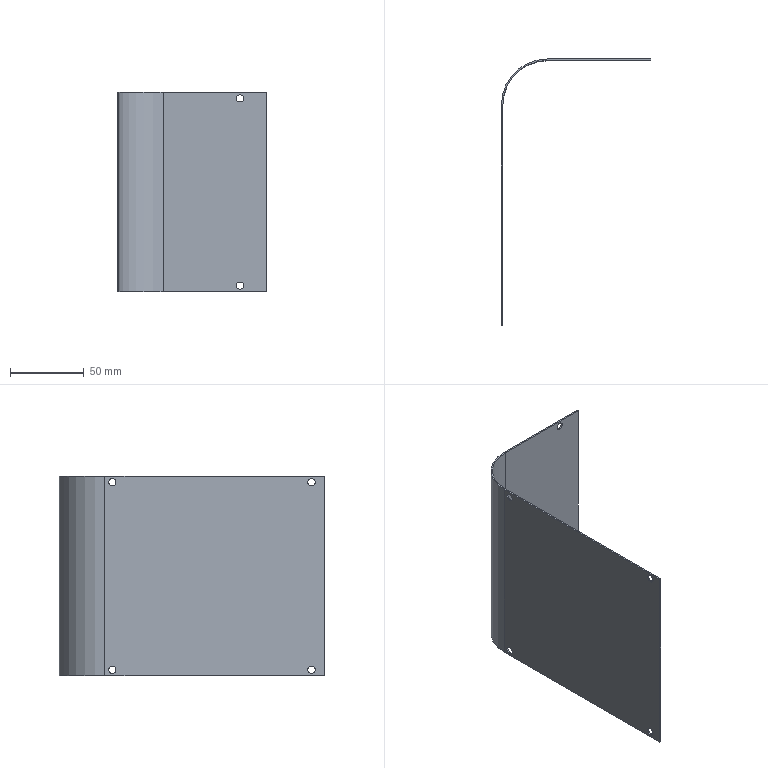Part | NX | 1 solid | 20 faces | box 101 x 180 x 135 mm | volume 35915 mm3 | plane 12 | cylinder 8 | commonest cylinder face diameters 5 x6 60 x1 62 x1
STEP:
#1=CARTESIAN_POINT('',(0.,-30.,67.5));
#2=VERTEX_POINT('',#1);
#3=CARTESIAN_POINT('',(-1.,-30.,67.5));
#4=VERTEX_POINT('',#3);
#5=CARTESIAN_POINT('',(0.,-30.,67.5));
#6=DIRECTION('',(-1.,0.,0.));
#7=VECTOR('',#6,1000.);
#8=LINE('',#5,#7);
#9=EDGE_CURVE('',#2,#4,#8,.T.);
#10=ORIENTED_EDGE('',*,*,#9,.F.);
#11=CARTESIAN_POINT('',(30.,0.,67.5));
#12=VERTEX_POINT('',#11);
#13=CARTESIAN_POINT('',(30.,-30.,67.5));
#14=DIRECTION('',(0.,0.,1.));
#15=DIRECTION('',(-1.,0.,0.));
#16=AXIS2_PLACEMENT_3D('',#13,#14,#15);
#17=CIRCLE('',#16,30.);
#18=EDGE_CURVE('',#12,#2,#17,.T.);
#19=ORIENTED_EDGE('',*,*,#18,.F.);
#20=CARTESIAN_POINT('',(30.,1.,67.5));
#21=VERTEX_POINT('',#20);
#22=CARTESIAN_POINT('',(30.,1.,67.5));
#23=DIRECTION('',(0.,-1.,0.));
#24=VECTOR('',#23,1000.);
#25=LINE('',#22,#24);
#26=EDGE_CURVE('',#21,#12,#25,.T.);
#27=ORIENTED_EDGE('',*,*,#26,.F.);
#28=CARTESIAN_POINT('',(30.,-30.,67.5));
#29=DIRECTION('',(0.,0.,1.));
#30=DIRECTION('',(1.,0.,0.));
#31=AXIS2_PLACEMENT_3D('',#28,#29,#30);
#32=CIRCLE('',#31,31.);
#33=EDGE_CURVE('',#21,#4,#32,.T.);
#34=ORIENTED_EDGE('',*,*,#33,.T.);
#35=EDGE_LOOP('',(#10,#19,#27,#34));
#36=FACE_BOUND('',#35,.T.);
#37=CARTESIAN_POINT('',(0.,-30.,67.5));
#38=DIRECTION('',(0.,0.,1.));
#39=DIRECTION('',(1.,0.,0.));
#40=AXIS2_PLACEMENT_3D('',#37,#38,#39);
#41=PLANE('',#40);
#42=ADVANCED_FACE('',(#36),#41,.T.);
#43=CARTESIAN_POINT('',(0.,-179.,67.5));
#44=VERTEX_POINT('',#43);
#45=CARTESIAN_POINT('',(0.,-30.,67.5));
#46=DIRECTION('',(0.,-1.,0.));
#47=VECTOR('',#46,1000.);
#48=LINE('',#45,#47);
#49=EDGE_CURVE('',#2,#44,#48,.T.);
#50=ORIENTED_EDGE('',*,*,#49,.F.);
#51=ORIENTED_EDGE('',*,*,#9,.T.);
#52=CARTESIAN_POINT('',(-1.,-179.,67.5));
#53=VERTEX_POINT('',#52);
#54=CARTESIAN_POINT('',(-1.,-30.,67.5));
#55=DIRECTION('',(0.,-1.,0.));
#56=VECTOR('',#55,1000.);
#57=LINE('',#54,#56);
#58=EDGE_CURVE('',#4,#53,#57,.T.);
#59=ORIENTED_EDGE('',*,*,#58,.T.);
#60=CARTESIAN_POINT('',(0.,-179.,67.5));
#61=DIRECTION('',(-1.,0.,0.));
#62=VECTOR('',#61,1000.);
#63=LINE('',#60,#62);
#64=EDGE_CURVE('',#44,#53,#63,.T.);
#65=ORIENTED_EDGE('',*,*,#64,.F.);
#66=EDGE_LOOP('',(#50,#51,#59,#65));
#67=FACE_BOUND('',#66,.T.);
#68=CARTESIAN_POINT('',(30.,1.,67.5));
#69=DIRECTION('',(0.,0.,1.));
#70=DIRECTION('',(1.,0.,0.));
#71=AXIS2_PLACEMENT_3D('',#68,#69,#70);
#72=PLANE('',#71);
#73=ADVANCED_FACE('',(#67),#72,.T.);
#74=CARTESIAN_POINT('',(30.,0.,-67.5));
#75=VERTEX_POINT('',#74);
#76=CARTESIAN_POINT('',(30.,1.,-67.5));
#77=VERTEX_POINT('',#76);
#78=CARTESIAN_POINT('',(30.,0.,-67.5));
#79=DIRECTION('',(0.,1.,0.));
#80=VECTOR('',#79,1000.);
#81=LINE('',#78,#80);
#82=EDGE_CURVE('',#75,#77,#81,.T.);
#83=ORIENTED_EDGE('',*,*,#82,.F.);
#84=CARTESIAN_POINT('',(0.,-30.,-67.5));
#85=VERTEX_POINT('',#84);
#86=CARTESIAN_POINT('',(30.,-30.,-67.5));
#87=DIRECTION('',(0.,0.,1.));
#88=DIRECTION('',(-1.,0.,0.));
#89=AXIS2_PLACEMENT_3D('',#86,#87,#88);
#90=CIRCLE('',#89,30.);
#91=EDGE_CURVE('',#75,#85,#90,.T.);
#92=ORIENTED_EDGE('',*,*,#91,.T.);
#93=CARTESIAN_POINT('',(-1.,-30.,-67.5));
#94=VERTEX_POINT('',#93);
#95=CARTESIAN_POINT('',(-1.,-30.,-67.5));
#96=DIRECTION('',(1.,0.,0.));
#97=VECTOR('',#96,1000.);
#98=LINE('',#95,#97);
#99=EDGE_CURVE('',#94,#85,#98,.T.);
#100=ORIENTED_EDGE('',*,*,#99,.F.);
#101=CARTESIAN_POINT('',(30.,-30.,-67.5));
#102=DIRECTION('',(0.,0.,1.));
#103=DIRECTION('',(1.,0.,0.));
#104=AXIS2_PLACEMENT_3D('',#101,#102,#103);
#105=CIRCLE('',#104,31.);
#106=EDGE_CURVE('',#77,#94,#105,.T.);
#107=ORIENTED_EDGE('',*,*,#106,.F.);
#108=EDGE_LOOP('',(#83,#92,#100,#107));
#109=FACE_BOUND('',#108,.T.);
#110=CARTESIAN_POINT('',(30.,0.,-67.5));
#111=DIRECTION('',(0.,0.,-1.));
#112=DIRECTION('',(-1.,0.,0.));
#113=AXIS2_PLACEMENT_3D('',#110,#111,#112);
#114=PLANE('',#113);
#115=ADVANCED_FACE('',(#109),#114,.T.);
#116=CARTESIAN_POINT('',(100.,0.,-67.5));
#117=VERTEX_POINT('',#116);
#118=CARTESIAN_POINT('',(30.,0.,-67.5));
#119=DIRECTION('',(-1.,0.,0.));
#120=VECTOR('',#119,1000.);
#121=LINE('',#118,#120);
#122=EDGE_CURVE('',#117,#75,#121,.T.);
#123=ORIENTED_EDGE('',*,*,#122,.T.);
#124=ORIENTED_EDGE('',*,*,#82,.T.);
#125=CARTESIAN_POINT('',(100.,1.,-67.5));
#126=VERTEX_POINT('',#125);
#127=CARTESIAN_POINT('',(30.,1.,-67.5));
#128=DIRECTION('',(1.,0.,0.));
#129=VECTOR('',#128,1000.);
#130=LINE('',#127,#129);
#131=EDGE_CURVE('',#126,#77,#130,.F.);
#132=ORIENTED_EDGE('',*,*,#131,.F.);
#133=CARTESIAN_POINT('',(100.,1.,-67.5));
#134=DIRECTION('',(0.,-1.,0.));
#135=VECTOR('',#134,1000.);
#136=LINE('',#133,#135);
#137=EDGE_CURVE('',#126,#117,#136,.T.);
#138=ORIENTED_EDGE('',*,*,#137,.T.);
#139=EDGE_LOOP('',(#123,#124,#132,#138));
#140=FACE_BOUND('',#139,.T.);
#141=CARTESIAN_POINT('',(-1.,-30.,-67.5));
#142=DIRECTION('',(0.,0.,-1.));
#143=DIRECTION('',(-1.,0.,0.));
#144=AXIS2_PLACEMENT_3D('',#141,#142,#143);
#145=PLANE('',#144);
#146=ADVANCED_FACE('',(#140),#145,.T.);
#147=CARTESIAN_POINT('',(-1.,-32.5,63.5));
#148=VERTEX_POINT('',#147);
#149=CARTESIAN_POINT('',(-1.,-35.,63.5));
#150=DIRECTION('',(-1.,0.,0.));
#151=DIRECTION('',(0.,1.,0.));
#152=AXIS2_PLACEMENT_3D('',#149,#150,#151);
#153=CIRCLE('',#152,2.5);
#154=EDGE_CURVE('',#148,#148,#153,.T.);
#155=ORIENTED_EDGE('',*,*,#154,.F.);
#156=EDGE_LOOP('',(#155));
#157=FACE_BOUND('',#156,.T.);
#158=CARTESIAN_POINT('',(-1.,-37.5,-63.5));
#159=VERTEX_POINT('',#158);
#160=CARTESIAN_POINT('',(-1.,-35.,-63.5));
#161=DIRECTION('',(-1.,0.,0.));
#162=DIRECTION('',(0.,-1.,0.));
#163=AXIS2_PLACEMENT_3D('',#160,#161,#162);
#164=CIRCLE('',#163,2.5);
#165=EDGE_CURVE('',#159,#159,#164,.T.);
#166=ORIENTED_EDGE('',*,*,#165,.F.);
#167=EDGE_LOOP('',(#166));
#168=FACE_BOUND('',#167,.T.);
#169=CARTESIAN_POINT('',(-1.,-172.5,63.5));
#170=VERTEX_POINT('',#169);
#171=CARTESIAN_POINT('',(-1.,-170.,63.5));
#172=DIRECTION('',(-1.,0.,0.));
#173=DIRECTION('',(0.,-1.,0.));
#174=AXIS2_PLACEMENT_3D('',#171,#172,#173);
#175=CIRCLE('',#174,2.5);
#176=EDGE_CURVE('',#170,#170,#175,.T.);
#177=ORIENTED_EDGE('',*,*,#176,.F.);
#178=EDGE_LOOP('',(#177));
#179=FACE_BOUND('',#178,.T.);
#180=CARTESIAN_POINT('',(-1.,-172.5,-63.5));
#181=VERTEX_POINT('',#180);
#182=CARTESIAN_POINT('',(-1.,-170.,-63.5));
#183=DIRECTION('',(-1.,0.,0.));
#184=DIRECTION('',(0.,-1.,0.));
#185=AXIS2_PLACEMENT_3D('',#182,#183,#184);
#186=CIRCLE('',#185,2.5);
#187=EDGE_CURVE('',#181,#181,#186,.T.);
#188=ORIENTED_EDGE('',*,*,#187,.F.);
#189=EDGE_LOOP('',(#188));
#190=FACE_BOUND('',#189,.T.);
#191=CARTESIAN_POINT('',(-1.,-179.,-67.5));
#192=VERTEX_POINT('',#191);
#193=CARTESIAN_POINT('',(-1.,-30.,-67.5));
#194=DIRECTION('',(0.,-1.,0.));
#195=VECTOR('',#194,1000.);
#196=LINE('',#193,#195);
#197=EDGE_CURVE('',#94,#192,#196,.T.);
#198=ORIENTED_EDGE('',*,*,#197,.T.);
#199=CARTESIAN_POINT('',(-1.,-179.,67.5));
#200=DIRECTION('',(0.,0.,-1.));
#201=VECTOR('',#200,1000.);
#202=LINE('',#199,#201);
#203=EDGE_CURVE('',#53,#192,#202,.T.);
#204=ORIENTED_EDGE('',*,*,#203,.F.);
#205=ORIENTED_EDGE('',*,*,#58,.F.);
#206=CARTESIAN_POINT('',(-1.,-30.,67.5));
#207=DIRECTION('',(0.,0.,-1.));
#208=VECTOR('',#207,1000.);
#209=LINE('',#206,#208);
#210=EDGE_CURVE('',#4,#94,#209,.T.);
#211=ORIENTED_EDGE('',*,*,#210,.T.);
#212=EDGE_LOOP('',(#198,#204,#205,#211));
#213=FACE_BOUND('',#212,.T.);
#214=CARTESIAN_POINT('',(-1.,-30.,67.5));
#215=DIRECTION('',(1.,0.,0.));
#216=DIRECTION('',(0.,1.,0.));
#217=AXIS2_PLACEMENT_3D('',#214,#215,#216);
#218=PLANE('',#217);
#219=ADVANCED_FACE('',(#157,#168,#179,#190,#213),#218,.F.);
#220=CARTESIAN_POINT('',(0.,-179.,-67.5));
#221=VERTEX_POINT('',#220);
#222=CARTESIAN_POINT('',(0.,-179.,-67.5));
#223=DIRECTION('',(-1.,0.,0.));
#224=VECTOR('',#223,1000.);
#225=LINE('',#222,#224);
#226=EDGE_CURVE('',#221,#192,#225,.T.);
#227=ORIENTED_EDGE('',*,*,#226,.F.);
#228=CARTESIAN_POINT('',(0.,-179.,67.5));
#229=DIRECTION('',(0.,0.,-1.));
#230=VECTOR('',#229,1000.);
#231=LINE('',#228,#230);
#232=EDGE_CURVE('',#44,#221,#231,.T.);
#233=ORIENTED_EDGE('',*,*,#232,.F.);
#234=ORIENTED_EDGE('',*,*,#64,.T.);
#235=ORIENTED_EDGE('',*,*,#203,.T.);
#236=EDGE_LOOP('',(#227,#233,#234,#235));
#237=FACE_BOUND('',#236,.T.);
#238=CARTESIAN_POINT('',(0.,-179.,67.5));
#239=DIRECTION('',(0.,-1.,0.));
#240=DIRECTION('',(0.,0.,-1.));
#241=AXIS2_PLACEMENT_3D('',#238,#239,#240);
#242=PLANE('',#241);
#243=ADVANCED_FACE('',(#237),#242,.T.);
#244=CARTESIAN_POINT('',(0.,-32.5,63.5));
#245=VERTEX_POINT('',#244);
#246=CARTESIAN_POINT('',(0.,-35.,63.5));
#247=DIRECTION('',(1.,0.,0.));
#248=DIRECTION('',(0.,1.,0.));
#249=AXIS2_PLACEMENT_3D('',#246,#247,#248);
#250=CIRCLE('',#249,2.5);
#251=EDGE_CURVE('',#245,#245,#250,.T.);
#252=ORIENTED_EDGE('',*,*,#251,.F.);
#253=EDGE_LOOP('',(#252));
#254=FACE_BOUND('',#253,.T.);
#255=CARTESIAN_POINT('',(0.,-32.5,-63.5));
#256=VERTEX_POINT('',#255);
#257=CARTESIAN_POINT('',(0.,-35.,-63.5));
#258=DIRECTION('',(1.,0.,0.));
#259=DIRECTION('',(0.,1.,0.));
#260=AXIS2_PLACEMENT_3D('',#257,#258,#259);
#261=CIRCLE('',#260,2.5);
#262=EDGE_CURVE('',#256,#256,#261,.T.);
#263=ORIENTED_EDGE('',*,*,#262,.F.);
#264=EDGE_LOOP('',(#263));
#265=FACE_BOUND('',#264,.T.);
#266=CARTESIAN_POINT('',(0.,-167.5,63.5));
#267=VERTEX_POINT('',#266);
#268=CARTESIAN_POINT('',(0.,-170.,63.5));
#269=DIRECTION('',(1.,0.,0.));
#270=DIRECTION('',(0.,1.,0.));
#271=AXIS2_PLACEMENT_3D('',#268,#269,#270);
#272=CIRCLE('',#271,2.5);
#273=EDGE_CURVE('',#267,#267,#272,.T.);
#274=ORIENTED_EDGE('',*,*,#273,.F.);
#275=EDGE_LOOP('',(#274));
#276=FACE_BOUND('',#275,.T.);
#277=CARTESIAN_POINT('',(0.,-167.5,-63.5));
#278=VERTEX_POINT('',#277);
#279=CARTESIAN_POINT('',(0.,-170.,-63.5));
#280=DIRECTION('',(1.,0.,0.));
#281=DIRECTION('',(0.,1.,0.));
#282=AXIS2_PLACEMENT_3D('',#279,#280,#281);
#283=CIRCLE('',#282,2.5);
#284=EDGE_CURVE('',#278,#278,#283,.T.);
#285=ORIENTED_EDGE('',*,*,#284,.F.);
#286=EDGE_LOOP('',(#285));
#287=FACE_BOUND('',#286,.T.);
#288=CARTESIAN_POINT('',(0.,-30.,-67.5));
#289=DIRECTION('',(0.,-1.,0.));
#290=VECTOR('',#289,1000.);
#291=LINE('',#288,#290);
#292=EDGE_CURVE('',#85,#221,#291,.T.);
#293=ORIENTED_EDGE('',*,*,#292,.F.);
#294=CARTESIAN_POINT('',(0.,-30.,67.5));
#295=DIRECTION('',(0.,0.,-1.));
#296=VECTOR('',#295,1000.);
#297=LINE('',#294,#296);
#298=EDGE_CURVE('',#2,#85,#297,.T.);
#299=ORIENTED_EDGE('',*,*,#298,.F.);
#300=ORIENTED_EDGE('',*,*,#49,.T.);
#301=ORIENTED_EDGE('',*,*,#232,.T.);
#302=EDGE_LOOP('',(#293,#299,#300,#301));
#303=FACE_BOUND('',#302,.T.);
#304=CARTESIAN_POINT('',(0.,-30.,67.5));
#305=DIRECTION('',(1.,0.,0.));
#306=DIRECTION('',(0.,1.,0.));
#307=AXIS2_PLACEMENT_3D('',#304,#305,#306);
#308=PLANE('',#307);
#309=ADVANCED_FACE('',(#254,#265,#276,#287,#303),#308,.T.);
#310=ORIENTED_EDGE('',*,*,#91,.F.);
#311=CARTESIAN_POINT('',(30.,0.,67.5));
#312=DIRECTION('',(0.,0.,-1.));
#313=VECTOR('',#312,1000.);
#314=LINE('',#311,#313);
#315=EDGE_CURVE('',#12,#75,#314,.T.);
#316=ORIENTED_EDGE('',*,*,#315,.F.);
#317=ORIENTED_EDGE('',*,*,#18,.T.);
#318=ORIENTED_EDGE('',*,*,#298,.T.);
#319=EDGE_LOOP('',(#310,#316,#317,#318));
#320=FACE_BOUND('',#319,.T.);
#321=CARTESIAN_POINT('',(30.,-30.,67.5));
#322=DIRECTION('',(0.,0.,-1.));
#323=DIRECTION('',(-1.,0.,0.));
#324=AXIS2_PLACEMENT_3D('',#321,#322,#323);
#325=CYLINDRICAL_SURFACE('',#324,30.);
#326=ADVANCED_FACE('',(#320),#325,.F.);
#327=CARTESIAN_POINT('',(82.,0.,61.));
#328=VERTEX_POINT('',#327);
#329=CARTESIAN_POINT('',(82.,0.,63.5));
#330=DIRECTION('',(0.,-1.,0.));
#331=DIRECTION('',(0.,0.,-1.));
#332=AXIS2_PLACEMENT_3D('',#329,#330,#331);
#333=CIRCLE('',#332,2.5);
#334=EDGE_CURVE('',#328,#328,#333,.T.);
#335=ORIENTED_EDGE('',*,*,#334,.F.);
#336=EDGE_LOOP('',(#335));
#337=FACE_BOUND('',#336,.T.);
#338=CARTESIAN_POINT('',(82.,0.,-66.));
#339=VERTEX_POINT('',#338);
#340=CARTESIAN_POINT('',(82.,0.,-63.5));
#341=DIRECTION('',(0.,-1.,0.));
#342=DIRECTION('',(0.,0.,-1.));
#343=AXIS2_PLACEMENT_3D('',#340,#341,#342);
#344=CIRCLE('',#343,2.5);
#345=EDGE_CURVE('',#339,#339,#344,.T.);
#346=ORIENTED_EDGE('',*,*,#345,.F.);
#347=EDGE_LOOP('',(#346));
#348=FACE_BOUND('',#347,.T.);
#349=ORIENTED_EDGE('',*,*,#122,.F.);
#350=CARTESIAN_POINT('',(100.,0.,67.5));
#351=VERTEX_POINT('',#350);
#352=CARTESIAN_POINT('',(100.,0.,67.5));
#353=DIRECTION('',(0.,0.,-1.));
#354=VECTOR('',#353,1000.);
#355=LINE('',#352,#354);
#356=EDGE_CURVE('',#351,#117,#355,.T.);
#357=ORIENTED_EDGE('',*,*,#356,.F.);
#358=CARTESIAN_POINT('',(30.,0.,67.5));
#359=DIRECTION('',(-1.,0.,0.));
#360=VECTOR('',#359,1000.);
#361=LINE('',#358,#360);
#362=EDGE_CURVE('',#351,#12,#361,.T.);
#363=ORIENTED_EDGE('',*,*,#362,.T.);
#364=ORIENTED_EDGE('',*,*,#315,.T.);
#365=EDGE_LOOP('',(#349,#357,#363,#364));
#366=FACE_BOUND('',#365,.T.);
#367=CARTESIAN_POINT('',(30.,0.,67.5));
#368=DIRECTION('',(0.,-1.,0.));
#369=DIRECTION('',(0.,0.,-1.));
#370=AXIS2_PLACEMENT_3D('',#367,#368,#369);
#371=PLANE('',#370);
#372=ADVANCED_FACE('',(#337,#348,#366),#371,.T.);
#373=ORIENTED_EDGE('',*,*,#137,.F.);
#374=CARTESIAN_POINT('',(100.,1.,67.5));
#375=VERTEX_POINT('',#374);
#376=CARTESIAN_POINT('',(100.,1.,67.5));
#377=DIRECTION('',(0.,0.,-1.));
#378=VECTOR('',#377,1000.);
#379=LINE('',#376,#378);
#380=EDGE_CURVE('',#375,#126,#379,.T.);
#381=ORIENTED_EDGE('',*,*,#380,.F.);
#382=CARTESIAN_POINT('',(100.,1.,67.5));
#383=DIRECTION('',(0.,-1.,0.));
#384=VECTOR('',#383,1000.);
#385=LINE('',#382,#384);
#386=EDGE_CURVE('',#375,#351,#385,.T.);
#387=ORIENTED_EDGE('',*,*,#386,.T.);
#388=ORIENTED_EDGE('',*,*,#356,.T.);
#389=EDGE_LOOP('',(#373,#381,#387,#388));
#390=FACE_BOUND('',#389,.T.);
#391=CARTESIAN_POINT('',(100.,1.,67.5));
#392=DIRECTION('',(1.,0.,0.));
#393=DIRECTION('',(0.,0.,-1.));
#394=AXIS2_PLACEMENT_3D('',#391,#392,#393);
#395=PLANE('',#394);
#396=ADVANCED_FACE('',(#390),#395,.T.);
#397=CARTESIAN_POINT('',(82.,1.,66.));
#398=VERTEX_POINT('',#397);
#399=CARTESIAN_POINT('',(82.,1.,63.5));
#400=DIRECTION('',(0.,1.,0.));
#401=DIRECTION('',(0.,0.,1.));
#402=AXIS2_PLACEMENT_3D('',#399,#400,#401);
#403=CIRCLE('',#402,2.5);
#404=EDGE_CURVE('',#398,#398,#403,.T.);
#405=ORIENTED_EDGE('',*,*,#404,.F.);
#406=EDGE_LOOP('',(#405));
#407=FACE_BOUND('',#406,.T.);
#408=CARTESIAN_POINT('',(82.,1.,-61.));
#409=VERTEX_POINT('',#408);
#410=CARTESIAN_POINT('',(82.,1.,-63.5));
#411=DIRECTION('',(0.,1.,0.));
#412=DIRECTION('',(0.,0.,1.));
#413=AXIS2_PLACEMENT_3D('',#410,#411,#412);
#414=CIRCLE('',#413,2.5);
#415=EDGE_CURVE('',#409,#409,#414,.T.);
#416=ORIENTED_EDGE('',*,*,#415,.F.);
#417=EDGE_LOOP('',(#416));
#418=FACE_BOUND('',#417,.T.);
#419=ORIENTED_EDGE('',*,*,#131,.T.);
#420=CARTESIAN_POINT('',(30.,1.,67.5));
#421=DIRECTION('',(0.,0.,-1.));
#422=VECTOR('',#421,1000.);
#423=LINE('',#420,#422);
#424=EDGE_CURVE('',#21,#77,#423,.T.);
#425=ORIENTED_EDGE('',*,*,#424,.F.);
#426=CARTESIAN_POINT('',(30.,1.,67.5));
#427=DIRECTION('',(1.,0.,0.));
#428=VECTOR('',#427,1000.);
#429=LINE('',#426,#428);
#430=EDGE_CURVE('',#375,#21,#429,.F.);
#431=ORIENTED_EDGE('',*,*,#430,.F.);
#432=ORIENTED_EDGE('',*,*,#380,.T.);
#433=EDGE_LOOP('',(#419,#425,#431,#432));
#434=FACE_BOUND('',#433,.T.);
#435=CARTESIAN_POINT('',(30.,1.,67.5));
#436=DIRECTION('',(0.,-1.,0.));
#437=DIRECTION('',(0.,0.,-1.));
#438=AXIS2_PLACEMENT_3D('',#435,#436,#437);
#439=PLANE('',#438);
#440=ADVANCED_FACE('',(#407,#418,#434),#439,.F.);
#441=ORIENTED_EDGE('',*,*,#106,.T.);
#442=ORIENTED_EDGE('',*,*,#210,.F.);
#443=ORIENTED_EDGE('',*,*,#33,.F.);
#444=ORIENTED_EDGE('',*,*,#424,.T.);
#445=EDGE_LOOP('',(#441,#442,#443,#444));
#446=FACE_BOUND('',#445,.T.);
#447=CARTESIAN_POINT('',(30.,-30.,67.5));
#448=DIRECTION('',(0.,0.,-1.));
#449=DIRECTION('',(-1.,0.,0.));
#450=AXIS2_PLACEMENT_3D('',#447,#448,#449);
#451=CYLINDRICAL_SURFACE('',#450,31.);
#452=ADVANCED_FACE('',(#446),#451,.T.);
#453=ORIENTED_EDGE('',*,*,#430,.T.);
#454=ORIENTED_EDGE('',*,*,#26,.T.);
#455=ORIENTED_EDGE('',*,*,#362,.F.);
#456=ORIENTED_EDGE('',*,*,#386,.F.);
#457=EDGE_LOOP('',(#453,#454,#455,#456));
#458=FACE_BOUND('',#457,.T.);
#459=CARTESIAN_POINT('',(30.,-30.,67.5));
#460=DIRECTION('',(0.,0.,1.));
#461=DIRECTION('',(1.,0.,0.));
#462=AXIS2_PLACEMENT_3D('',#459,#460,#461);
#463=PLANE('',#462);
#464=ADVANCED_FACE('',(#458),#463,.T.);
#465=ORIENTED_EDGE('',*,*,#197,.F.);
#466=ORIENTED_EDGE('',*,*,#99,.T.);
#467=ORIENTED_EDGE('',*,*,#292,.T.);
#468=ORIENTED_EDGE('',*,*,#226,.T.);
#469=EDGE_LOOP('',(#465,#466,#467,#468));
#470=FACE_BOUND('',#469,.T.);
#471=CARTESIAN_POINT('',(30.,-30.,-67.5));
#472=DIRECTION('',(0.,0.,1.));
#473=DIRECTION('',(1.,0.,0.));
#474=AXIS2_PLACEMENT_3D('',#471,#472,#473);
#475=PLANE('',#474);
#476=ADVANCED_FACE('',(#470),#475,.F.);
#477=ORIENTED_EDGE('',*,*,#345,.T.);
#478=EDGE_LOOP('',(#477));
#479=FACE_BOUND('',#478,.T.);
#480=ORIENTED_EDGE('',*,*,#415,.T.);
#481=EDGE_LOOP('',(#480));
#482=FACE_BOUND('',#481,.T.);
#483=CARTESIAN_POINT('',(82.,-179.,-63.5));
#484=DIRECTION('',(0.,1.,0.));
#485=DIRECTION('',(0.,0.,1.));
#486=AXIS2_PLACEMENT_3D('',#483,#484,#485);
#487=CYLINDRICAL_SURFACE('',#486,2.5);
#488=ADVANCED_FACE('',(#479,#482),#487,.F.);
#489=ORIENTED_EDGE('',*,*,#334,.T.);
#490=EDGE_LOOP('',(#489));
#491=FACE_BOUND('',#490,.T.);
#492=ORIENTED_EDGE('',*,*,#404,.T.);
#493=EDGE_LOOP('',(#492));
#494=FACE_BOUND('',#493,.T.);
#495=CARTESIAN_POINT('',(82.,-179.,63.5));
#496=DIRECTION('',(0.,1.,0.));
#497=DIRECTION('',(0.,0.,1.));
#498=AXIS2_PLACEMENT_3D('',#495,#496,#497);
#499=CYLINDRICAL_SURFACE('',#498,2.5);
#500=ADVANCED_FACE('',(#491,#494),#499,.F.);
#501=ORIENTED_EDGE('',*,*,#284,.T.);
#502=EDGE_LOOP('',(#501));
#503=FACE_BOUND('',#502,.T.);
#504=ORIENTED_EDGE('',*,*,#187,.T.);
#505=EDGE_LOOP('',(#504));
#506=FACE_BOUND('',#505,.T.);
#507=CARTESIAN_POINT('',(100.,-170.,-63.5));
#508=DIRECTION('',(-1.,0.,0.));
#509=DIRECTION('',(0.,-1.,0.));
#510=AXIS2_PLACEMENT_3D('',#507,#508,#509);
#511=CYLINDRICAL_SURFACE('',#510,2.5);
#512=ADVANCED_FACE('',(#503,#506),#511,.F.);
#513=ORIENTED_EDGE('',*,*,#273,.T.);
#514=EDGE_LOOP('',(#513));
#515=FACE_BOUND('',#514,.T.);
#516=ORIENTED_EDGE('',*,*,#176,.T.);
#517=EDGE_LOOP('',(#516));
#518=FACE_BOUND('',#517,.T.);
#519=CARTESIAN_POINT('',(100.,-170.,63.5));
#520=DIRECTION('',(-1.,0.,0.));
#521=DIRECTION('',(0.,-1.,0.));
#522=AXIS2_PLACEMENT_3D('',#519,#520,#521);
#523=CYLINDRICAL_SURFACE('',#522,2.5);
#524=ADVANCED_FACE('',(#515,#518),#523,.F.);
#525=ORIENTED_EDGE('',*,*,#262,.T.);
#526=EDGE_LOOP('',(#525));
#527=FACE_BOUND('',#526,.T.);
#528=ORIENTED_EDGE('',*,*,#165,.T.);
#529=EDGE_LOOP('',(#528));
#530=FACE_BOUND('',#529,.T.);
#531=CARTESIAN_POINT('',(100.,-35.,-63.5));
#532=DIRECTION('',(-1.,0.,0.));
#533=DIRECTION('',(0.,-1.,0.));
#534=AXIS2_PLACEMENT_3D('',#531,#532,#533);
#535=CYLINDRICAL_SURFACE('',#534,2.5);
#536=ADVANCED_FACE('',(#527,#530),#535,.F.);
#537=ORIENTED_EDGE('',*,*,#251,.T.);
#538=EDGE_LOOP('',(#537));
#539=FACE_BOUND('',#538,.T.);
#540=ORIENTED_EDGE('',*,*,#154,.T.);
#541=EDGE_LOOP('',(#540));
#542=FACE_BOUND('',#541,.T.);
#543=CARTESIAN_POINT('',(100.,-35.,63.5));
#544=DIRECTION('',(-1.,0.,0.));
#545=DIRECTION('',(0.,-1.,0.));
#546=AXIS2_PLACEMENT_3D('',#543,#544,#545);
#547=CYLINDRICAL_SURFACE('',#546,2.5);
#548=ADVANCED_FACE('',(#539,#542),#547,.F.);
#549=CLOSED_SHELL('',(#42,#73,#115,#146,#219,#243,#309,#326,#372,#396,#440,#452,#464,#476,#488,#500,#512,#524,#536,#548));
#550=MANIFOLD_SOLID_BREP('',#549);
#551=(LENGTH_UNIT()NAMED_UNIT(*)SI_UNIT(.MILLI.,.METRE.));
#552=UNCERTAINTY_MEASURE_WITH_UNIT(LENGTH_MEASURE(0.00001),#551,'','');
#553=(NAMED_UNIT(*)PLANE_ANGLE_UNIT()SI_UNIT($,.RADIAN.));
#554=(NAMED_UNIT(*)SI_UNIT($,.STERADIAN.)SOLID_ANGLE_UNIT());
#555=(GEOMETRIC_REPRESENTATION_CONTEXT(3)GLOBAL_UNCERTAINTY_ASSIGNED_CONTEXT((#552))GLOBAL_UNIT_ASSIGNED_CONTEXT((#551,#553,#554))REPRESENTATION_CONTEXT('',''));
#556=ADVANCED_BREP_SHAPE_REPRESENTATION('',(#550),#555);